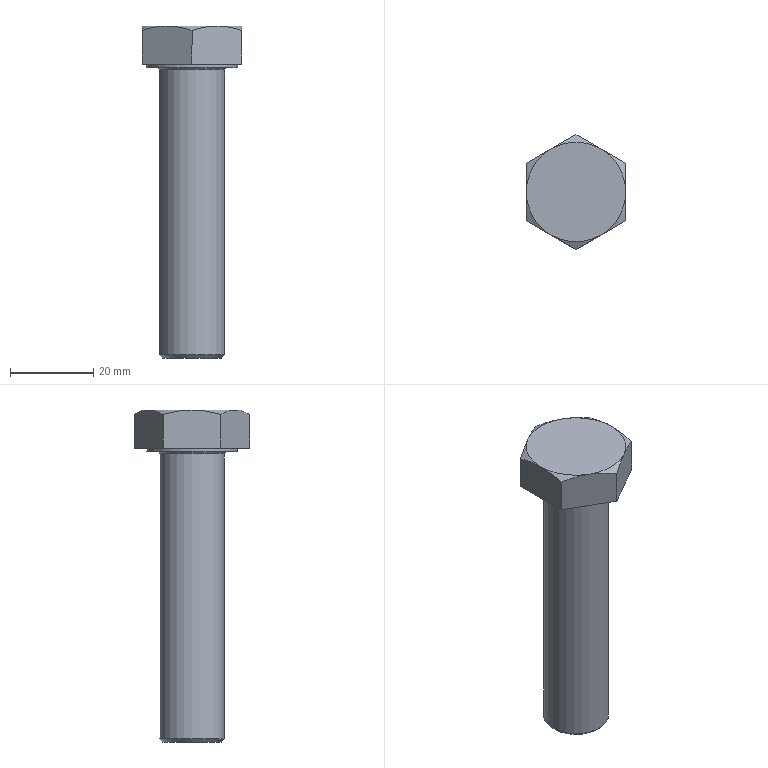Part | NX | features SKETCH 4, EXTRUDE 3, META 3, DATUM_CSYS 2, BLEND 1, CHAMFER 1, LINE 1, SWP104 1, SYMBOLIC_THREAD 1, THREADS 1 | 1 solid | 20 faces | box 24 x 27.713 x 80 mm | volume 18388 mm3 | plane 10 | cone 7 | cylinder 2 | torus 1 | commonest cylinder face diameters 15.682 x1 22 x1
STEP:
#1=CARTESIAN_POINT('',(8.441,0.,0.));
#2=VERTEX_POINT('',#1);
#3=CARTESIAN_POINT('',(0.,0.,0.));
#4=DIRECTION('',(0.,0.,1.));
#5=DIRECTION('',(1.,0.,0.));
#6=AXIS2_PLACEMENT_3D('',#3,#4,#5);
#7=CIRCLE('',#6,8.441);
#8=EDGE_CURVE('',#2,#2,#7,.T.);
#9=ORIENTED_EDGE('',*,*,#8,.T.);
#10=EDGE_LOOP('',(#9));
#11=FACE_BOUND('',#10,.T.);
#12=CARTESIAN_POINT('',(11.,0.,0.));
#13=VERTEX_POINT('',#12);
#14=CARTESIAN_POINT('',(0.,0.,0.));
#15=DIRECTION('',(0.,0.,1.));
#16=DIRECTION('',(1.,0.,0.));
#17=AXIS2_PLACEMENT_3D('',#14,#15,#16);
#18=CIRCLE('',#17,11.);
#19=EDGE_CURVE('',#13,#13,#18,.T.);
#20=ORIENTED_EDGE('',*,*,#19,.F.);
#21=EDGE_LOOP('',(#20));
#22=FACE_BOUND('',#21,.T.);
#23=CARTESIAN_POINT('',(0.,0.,0.));
#24=DIRECTION('',(0.,0.,1.));
#25=DIRECTION('',(1.,0.,0.));
#26=AXIS2_PLACEMENT_3D('',#23,#24,#25);
#27=PLANE('',#26);
#28=ADVANCED_FACE('',(#11,#22),#27,.F.);
#29=CARTESIAN_POINT('',(12.,6.928,8.928));
#30=VERTEX_POINT('',#29);
#31=CARTESIAN_POINT('',(6.,10.392,10.));
#32=VERTEX_POINT('',#31);
#33=CARTESIAN_POINT('',(12.,6.928,8.928));
#34=CARTESIAN_POINT('',(10.037,8.062,9.583));
#35=CARTESIAN_POINT('',(8.044,9.212,10.));
#36=CARTESIAN_POINT('',(6.,10.392,10.));
#37=B_SPLINE_CURVE_WITH_KNOTS('',3,(#33,#34,#35,#36),.UNSPECIFIED.,.F.,.F.,(4,4),(0.000000238,0.00701),.UNSPECIFIED.);
#38=EDGE_CURVE('',#30,#32,#37,.T.);
#39=ORIENTED_EDGE('',*,*,#38,.F.);
#40=CARTESIAN_POINT('',(12.,6.928,0.8));
#41=VERTEX_POINT('',#40);
#42=CARTESIAN_POINT('',(12.,6.928,10.));
#43=DIRECTION('',(0.,0.,-1.));
#44=VECTOR('',#43,1000.);
#45=LINE('',#42,#44);
#46=EDGE_CURVE('',#30,#41,#45,.T.);
#47=ORIENTED_EDGE('',*,*,#46,.T.);
#48=CARTESIAN_POINT('',(0.,13.856,0.8));
#49=VERTEX_POINT('',#48);
#50=CARTESIAN_POINT('',(0.,13.856,0.8));
#51=DIRECTION('',(0.866,-0.5,0.));
#52=VECTOR('',#51,1000.);
#53=LINE('',#50,#52);
#54=EDGE_CURVE('',#49,#41,#53,.T.);
#55=ORIENTED_EDGE('',*,*,#54,.F.);
#56=CARTESIAN_POINT('',(0.,13.856,8.928));
#57=VERTEX_POINT('',#56);
#58=CARTESIAN_POINT('',(0.,13.856,10.));
#59=DIRECTION('',(0.,0.,-1.));
#60=VECTOR('',#59,1000.);
#61=LINE('',#58,#60);
#62=EDGE_CURVE('',#57,#49,#61,.T.);
#63=ORIENTED_EDGE('',*,*,#62,.F.);
#64=CARTESIAN_POINT('',(6.,10.392,10.));
#65=CARTESIAN_POINT('',(3.963,11.568,10.));
#66=CARTESIAN_POINT('',(1.958,12.726,9.581));
#67=CARTESIAN_POINT('',(0.,13.856,8.928));
#68=B_SPLINE_CURVE_WITH_KNOTS('',3,(#64,#65,#66,#67),.UNSPECIFIED.,.F.,.F.,(4,4),(0.00701,0.01399),.UNSPECIFIED.);
#69=EDGE_CURVE('',#32,#57,#68,.T.);
#70=ORIENTED_EDGE('',*,*,#69,.F.);
#71=EDGE_LOOP('',(#39,#47,#55,#63,#70));
#72=FACE_BOUND('',#71,.T.);
#73=CARTESIAN_POINT('',(0.,13.856,10.));
#74=DIRECTION('',(0.5,0.866,0.));
#75=DIRECTION('',(-0.866,0.5,0.));
#76=AXIS2_PLACEMENT_3D('',#73,#74,#75);
#77=PLANE('',#76);
#78=ADVANCED_FACE('',(#72),#77,.T.);
#79=CARTESIAN_POINT('',(12.,-6.928,8.928));
#80=VERTEX_POINT('',#79);
#81=CARTESIAN_POINT('',(12.,0.,10.));
#82=VERTEX_POINT('',#81);
#83=CARTESIAN_POINT('',(12.,-6.928,8.928));
#84=CARTESIAN_POINT('',(12.,-4.675,9.579));
#85=CARTESIAN_POINT('',(12.,-2.342,10.));
#86=CARTESIAN_POINT('',(12.,0.,10.));
#87=B_SPLINE_CURVE_WITH_KNOTS('',3,(#83,#84,#85,#86),.UNSPECIFIED.,.F.,.F.,(4,4),(0.01236,0.01937),.UNSPECIFIED.);
#88=EDGE_CURVE('',#80,#82,#87,.T.);
#89=ORIENTED_EDGE('',*,*,#88,.F.);
#90=CARTESIAN_POINT('',(12.,-6.928,0.8));
#91=VERTEX_POINT('',#90);
#92=CARTESIAN_POINT('',(12.,-6.928,10.));
#93=DIRECTION('',(0.,0.,-1.));
#94=VECTOR('',#93,1000.);
#95=LINE('',#92,#94);
#96=EDGE_CURVE('',#80,#91,#95,.T.);
#97=ORIENTED_EDGE('',*,*,#96,.T.);
#98=CARTESIAN_POINT('',(12.,6.928,0.8));
#99=DIRECTION('',(0.,-1.,0.));
#100=VECTOR('',#99,1000.);
#101=LINE('',#98,#100);
#102=EDGE_CURVE('',#41,#91,#101,.T.);
#103=ORIENTED_EDGE('',*,*,#102,.F.);
#104=ORIENTED_EDGE('',*,*,#46,.F.);
#105=CARTESIAN_POINT('',(12.,0.,10.));
#106=CARTESIAN_POINT('',(12.,2.343,10.));
#107=CARTESIAN_POINT('',(12.,4.688,9.575));
#108=CARTESIAN_POINT('',(12.,6.928,8.928));
#109=B_SPLINE_CURVE_WITH_KNOTS('',3,(#105,#106,#107,#108),.UNSPECIFIED.,.F.,.F.,(4,4),(0.01937,0.02638),.UNSPECIFIED.);
#110=EDGE_CURVE('',#82,#30,#109,.T.);
#111=ORIENTED_EDGE('',*,*,#110,.F.);
#112=EDGE_LOOP('',(#89,#97,#103,#104,#111));
#113=FACE_BOUND('',#112,.T.);
#114=CARTESIAN_POINT('',(12.,6.928,10.));
#115=DIRECTION('',(1.,0.,0.));
#116=DIRECTION('',(0.,0.,-1.));
#117=AXIS2_PLACEMENT_3D('',#114,#115,#116);
#118=PLANE('',#117);
#119=ADVANCED_FACE('',(#113),#118,.T.);
#120=CARTESIAN_POINT('',(0.,-13.856,8.928));
#121=VERTEX_POINT('',#120);
#122=CARTESIAN_POINT('',(6.,-10.392,10.));
#123=VERTEX_POINT('',#122);
#124=CARTESIAN_POINT('',(0.,-13.856,8.928));
#125=CARTESIAN_POINT('',(1.963,-12.723,9.583));
#126=CARTESIAN_POINT('',(3.956,-11.573,10.));
#127=CARTESIAN_POINT('',(6.,-10.392,10.));
#128=B_SPLINE_CURVE_WITH_KNOTS('',3,(#124,#125,#126,#127),.UNSPECIFIED.,.F.,.F.,(4,4),(0.000000238,0.00701),.UNSPECIFIED.);
#129=EDGE_CURVE('',#121,#123,#128,.T.);
#130=ORIENTED_EDGE('',*,*,#129,.F.);
#131=CARTESIAN_POINT('',(0.,-13.856,0.8));
#132=VERTEX_POINT('',#131);
#133=CARTESIAN_POINT('',(0.,-13.856,10.));
#134=DIRECTION('',(0.,0.,-1.));
#135=VECTOR('',#134,1000.);
#136=LINE('',#133,#135);
#137=EDGE_CURVE('',#121,#132,#136,.T.);
#138=ORIENTED_EDGE('',*,*,#137,.T.);
#139=CARTESIAN_POINT('',(12.,-6.928,0.8));
#140=DIRECTION('',(-0.866,-0.5,0.));
#141=VECTOR('',#140,1000.);
#142=LINE('',#139,#141);
#143=EDGE_CURVE('',#91,#132,#142,.T.);
#144=ORIENTED_EDGE('',*,*,#143,.F.);
#145=ORIENTED_EDGE('',*,*,#96,.F.);
#146=CARTESIAN_POINT('',(6.,-10.392,10.));
#147=CARTESIAN_POINT('',(8.037,-9.216,10.));
#148=CARTESIAN_POINT('',(10.042,-8.059,9.581));
#149=CARTESIAN_POINT('',(12.,-6.928,8.928));
#150=B_SPLINE_CURVE_WITH_KNOTS('',3,(#146,#147,#148,#149),.UNSPECIFIED.,.F.,.F.,(4,4),(0.00701,0.01399),.UNSPECIFIED.);
#151=EDGE_CURVE('',#123,#80,#150,.T.);
#152=ORIENTED_EDGE('',*,*,#151,.F.);
#153=EDGE_LOOP('',(#130,#138,#144,#145,#152));
#154=FACE_BOUND('',#153,.T.);
#155=CARTESIAN_POINT('',(12.,-6.928,10.));
#156=DIRECTION('',(0.5,-0.866,0.));
#157=DIRECTION('',(0.866,0.5,0.));
#158=AXIS2_PLACEMENT_3D('',#155,#156,#157);
#159=PLANE('',#158);
#160=ADVANCED_FACE('',(#154),#159,.T.);
#161=CARTESIAN_POINT('',(-12.,-6.928,8.928));
#162=VERTEX_POINT('',#161);
#163=CARTESIAN_POINT('',(-6.,-10.392,10.));
#164=VERTEX_POINT('',#163);
#165=CARTESIAN_POINT('',(-12.,-6.928,8.928));
#166=CARTESIAN_POINT('',(-10.037,-8.062,9.583));
#167=CARTESIAN_POINT('',(-8.044,-9.212,10.));
#168=CARTESIAN_POINT('',(-6.,-10.392,10.));
#169=B_SPLINE_CURVE_WITH_KNOTS('',3,(#165,#166,#167,#168),.UNSPECIFIED.,.F.,.F.,(4,4),(0.000000238,0.00701),.UNSPECIFIED.);
#170=EDGE_CURVE('',#162,#164,#169,.T.);
#171=ORIENTED_EDGE('',*,*,#170,.F.);
#172=CARTESIAN_POINT('',(-12.,-6.928,0.8));
#173=VERTEX_POINT('',#172);
#174=CARTESIAN_POINT('',(-12.,-6.928,10.));
#175=DIRECTION('',(0.,0.,-1.));
#176=VECTOR('',#175,1000.);
#177=LINE('',#174,#176);
#178=EDGE_CURVE('',#162,#173,#177,.T.);
#179=ORIENTED_EDGE('',*,*,#178,.T.);
#180=CARTESIAN_POINT('',(0.,-13.856,0.8));
#181=DIRECTION('',(-0.866,0.5,0.));
#182=VECTOR('',#181,1000.);
#183=LINE('',#180,#182);
#184=EDGE_CURVE('',#132,#173,#183,.T.);
#185=ORIENTED_EDGE('',*,*,#184,.F.);
#186=ORIENTED_EDGE('',*,*,#137,.F.);
#187=CARTESIAN_POINT('',(-6.,-10.392,10.));
#188=CARTESIAN_POINT('',(-3.963,-11.568,10.));
#189=CARTESIAN_POINT('',(-1.958,-12.726,9.581));
#190=CARTESIAN_POINT('',(0.,-13.856,8.928));
#191=B_SPLINE_CURVE_WITH_KNOTS('',3,(#187,#188,#189,#190),.UNSPECIFIED.,.F.,.F.,(4,4),(0.00701,0.01399),.UNSPECIFIED.);
#192=EDGE_CURVE('',#164,#121,#191,.T.);
#193=ORIENTED_EDGE('',*,*,#192,.F.);
#194=EDGE_LOOP('',(#171,#179,#185,#186,#193));
#195=FACE_BOUND('',#194,.T.);
#196=CARTESIAN_POINT('',(0.,-13.856,10.));
#197=DIRECTION('',(-0.5,-0.866,0.));
#198=DIRECTION('',(0.866,-0.5,0.));
#199=AXIS2_PLACEMENT_3D('',#196,#197,#198);
#200=PLANE('',#199);
#201=ADVANCED_FACE('',(#195),#200,.T.);
#202=CARTESIAN_POINT('',(-12.,6.928,8.928));
#203=VERTEX_POINT('',#202);
#204=CARTESIAN_POINT('',(-12.,0.,10.));
#205=VERTEX_POINT('',#204);
#206=CARTESIAN_POINT('',(-12.,0.,10.));
#207=CARTESIAN_POINT('',(-12.,2.343,10.));
#208=CARTESIAN_POINT('',(-12.,4.688,9.575));
#209=CARTESIAN_POINT('',(-12.,6.928,8.928));
#210=B_SPLINE_CURVE_WITH_KNOTS('',3,(#206,#207,#208,#209),.UNSPECIFIED.,.F.,.F.,(4,4),(0.01937,0.02638),.UNSPECIFIED.);
#211=EDGE_CURVE('',#203,#205,#210,.F.);
#212=ORIENTED_EDGE('',*,*,#211,.F.);
#213=CARTESIAN_POINT('',(-12.,6.928,0.8));
#214=VERTEX_POINT('',#213);
#215=CARTESIAN_POINT('',(-12.,6.928,10.));
#216=DIRECTION('',(0.,0.,-1.));
#217=VECTOR('',#216,1000.);
#218=LINE('',#215,#217);
#219=EDGE_CURVE('',#203,#214,#218,.T.);
#220=ORIENTED_EDGE('',*,*,#219,.T.);
#221=CARTESIAN_POINT('',(-12.,-6.928,0.8));
#222=DIRECTION('',(0.,1.,0.));
#223=VECTOR('',#222,1000.);
#224=LINE('',#221,#223);
#225=EDGE_CURVE('',#173,#214,#224,.T.);
#226=ORIENTED_EDGE('',*,*,#225,.F.);
#227=ORIENTED_EDGE('',*,*,#178,.F.);
#228=CARTESIAN_POINT('',(-12.,-6.928,8.928));
#229=CARTESIAN_POINT('',(-12.,-4.675,9.579));
#230=CARTESIAN_POINT('',(-12.,-2.342,10.));
#231=CARTESIAN_POINT('',(-12.,0.,10.));
#232=B_SPLINE_CURVE_WITH_KNOTS('',3,(#228,#229,#230,#231),.UNSPECIFIED.,.F.,.F.,(4,4),(0.01236,0.01937),.UNSPECIFIED.);
#233=EDGE_CURVE('',#205,#162,#232,.F.);
#234=ORIENTED_EDGE('',*,*,#233,.F.);
#235=EDGE_LOOP('',(#212,#220,#226,#227,#234));
#236=FACE_BOUND('',#235,.T.);
#237=CARTESIAN_POINT('',(-12.,-6.928,10.));
#238=DIRECTION('',(-1.,0.,0.));
#239=DIRECTION('',(0.,0.,1.));
#240=AXIS2_PLACEMENT_3D('',#237,#238,#239);
#241=PLANE('',#240);
#242=ADVANCED_FACE('',(#236),#241,.T.);
#243=CARTESIAN_POINT('',(-6.,10.392,10.));
#244=VERTEX_POINT('',#243);
#245=CARTESIAN_POINT('',(0.,13.856,8.928));
#246=CARTESIAN_POINT('',(-1.963,12.723,9.583));
#247=CARTESIAN_POINT('',(-3.956,11.573,10.));
#248=CARTESIAN_POINT('',(-6.,10.392,10.));
#249=B_SPLINE_CURVE_WITH_KNOTS('',3,(#245,#246,#247,#248),.UNSPECIFIED.,.F.,.F.,(4,4),(0.000000238,0.00701),.UNSPECIFIED.);
#250=EDGE_CURVE('',#57,#244,#249,.T.);
#251=ORIENTED_EDGE('',*,*,#250,.F.);
#252=ORIENTED_EDGE('',*,*,#62,.T.);
#253=CARTESIAN_POINT('',(-12.,6.928,0.8));
#254=DIRECTION('',(0.866,0.5,0.));
#255=VECTOR('',#254,1000.);
#256=LINE('',#253,#255);
#257=EDGE_CURVE('',#214,#49,#256,.T.);
#258=ORIENTED_EDGE('',*,*,#257,.F.);
#259=ORIENTED_EDGE('',*,*,#219,.F.);
#260=CARTESIAN_POINT('',(-6.,10.392,10.));
#261=CARTESIAN_POINT('',(-8.037,9.216,10.));
#262=CARTESIAN_POINT('',(-10.042,8.059,9.581));
#263=CARTESIAN_POINT('',(-12.,6.928,8.928));
#264=B_SPLINE_CURVE_WITH_KNOTS('',3,(#260,#261,#262,#263),.UNSPECIFIED.,.F.,.F.,(4,4),(0.00701,0.01399),.UNSPECIFIED.);
#265=EDGE_CURVE('',#244,#203,#264,.T.);
#266=ORIENTED_EDGE('',*,*,#265,.F.);
#267=EDGE_LOOP('',(#251,#252,#258,#259,#266));
#268=FACE_BOUND('',#267,.T.);
#269=CARTESIAN_POINT('',(-12.,6.928,10.));
#270=DIRECTION('',(-0.5,0.866,0.));
#271=DIRECTION('',(-0.866,-0.5,0.));
#272=AXIS2_PLACEMENT_3D('',#269,#270,#271);
#273=PLANE('',#272);
#274=ADVANCED_FACE('',(#268),#273,.T.);
#275=CARTESIAN_POINT('',(11.,0.,0.8));
#276=VERTEX_POINT('',#275);
#277=CARTESIAN_POINT('',(0.,0.,0.8));
#278=DIRECTION('',(0.,0.,1.));
#279=DIRECTION('',(1.,0.,0.));
#280=AXIS2_PLACEMENT_3D('',#277,#278,#279);
#281=CIRCLE('',#280,11.);
#282=EDGE_CURVE('',#276,#276,#281,.T.);
#283=ORIENTED_EDGE('',*,*,#282,.T.);
#284=EDGE_LOOP('',(#283));
#285=FACE_BOUND('',#284,.T.);
#286=ORIENTED_EDGE('',*,*,#54,.T.);
#287=ORIENTED_EDGE('',*,*,#102,.T.);
#288=ORIENTED_EDGE('',*,*,#143,.T.);
#289=ORIENTED_EDGE('',*,*,#184,.T.);
#290=ORIENTED_EDGE('',*,*,#225,.T.);
#291=ORIENTED_EDGE('',*,*,#257,.T.);
#292=EDGE_LOOP('',(#286,#287,#288,#289,#290,#291));
#293=FACE_BOUND('',#292,.T.);
#294=CARTESIAN_POINT('',(0.,13.856,0.8));
#295=DIRECTION('',(0.,0.,1.));
#296=DIRECTION('',(1.,0.,0.));
#297=AXIS2_PLACEMENT_3D('',#294,#295,#296);
#298=PLANE('',#297);
#299=ADVANCED_FACE('',(#285,#293),#298,.F.);
#300=ORIENTED_EDGE('',*,*,#282,.F.);
#301=EDGE_LOOP('',(#300));
#302=FACE_BOUND('',#301,.T.);
#303=ORIENTED_EDGE('',*,*,#19,.T.);
#304=EDGE_LOOP('',(#303));
#305=FACE_BOUND('',#304,.T.);
#306=CARTESIAN_POINT('',(0.,0.,0.8));
#307=DIRECTION('',(0.,0.,-1.));
#308=DIRECTION('',(-1.,0.,0.));
#309=AXIS2_PLACEMENT_3D('',#306,#307,#308);
#310=CYLINDRICAL_SURFACE('',#309,11.);
#311=ADVANCED_FACE('',(#302,#305),#310,.T.);
#312=CARTESIAN_POINT('',(-7.841,0.,-69.216));
#313=VERTEX_POINT('',#312);
#314=CARTESIAN_POINT('',(0.,0.,-69.216));
#315=DIRECTION('',(0.,0.,-1.));
#316=DIRECTION('',(-1.,0.,0.));
#317=AXIS2_PLACEMENT_3D('',#314,#315,#316);
#318=CIRCLE('',#317,7.841);
#319=EDGE_CURVE('',#313,#313,#318,.F.);
#320=ORIENTED_EDGE('',*,*,#319,.T.);
#321=EDGE_LOOP('',(#320));
#322=FACE_BOUND('',#321,.T.);
#323=CARTESIAN_POINT('',(7.841,0.,-0.6));
#324=VERTEX_POINT('',#323);
#325=CARTESIAN_POINT('',(0.,0.,-0.6));
#326=DIRECTION('',(0.,0.,1.));
#327=DIRECTION('',(1.,0.,0.));
#328=AXIS2_PLACEMENT_3D('',#325,#326,#327);
#329=CIRCLE('',#328,7.841);
#330=EDGE_CURVE('',#324,#324,#329,.F.);
#331=ORIENTED_EDGE('',*,*,#330,.T.);
#332=EDGE_LOOP('',(#331));
#333=FACE_BOUND('',#332,.T.);
#334=CARTESIAN_POINT('',(0.,0.,-70.));
#335=DIRECTION('',(0.,0.,1.));
#336=DIRECTION('',(1.,0.,0.));
#337=AXIS2_PLACEMENT_3D('',#334,#335,#336);
#338=CYLINDRICAL_SURFACE('',#337,7.841);
#339=ADVANCED_FACE('',(#322,#333),#338,.T.);
#340=CARTESIAN_POINT('',(-7.057,0.,-70.));
#341=VERTEX_POINT('',#340);
#342=CARTESIAN_POINT('',(0.,0.,-70.));
#343=DIRECTION('',(0.,0.,-1.));
#344=DIRECTION('',(-1.,0.,0.));
#345=AXIS2_PLACEMENT_3D('',#342,#343,#344);
#346=CIRCLE('',#345,7.057);
#347=EDGE_CURVE('',#341,#341,#346,.T.);
#348=ORIENTED_EDGE('',*,*,#347,.T.);
#349=EDGE_LOOP('',(#348));
#350=FACE_BOUND('',#349,.T.);
#351=CARTESIAN_POINT('',(0.,0.,-70.));
#352=DIRECTION('',(0.,0.,-1.));
#353=DIRECTION('',(-1.,0.,0.));
#354=AXIS2_PLACEMENT_3D('',#351,#352,#353);
#355=PLANE('',#354);
#356=ADVANCED_FACE('',(#350),#355,.T.);
#357=ORIENTED_EDGE('',*,*,#211,.T.);
#358=CARTESIAN_POINT('',(0.,0.,10.));
#359=DIRECTION('',(0.,0.,-1.));
#360=DIRECTION('',(-1.,0.,0.));
#361=AXIS2_PLACEMENT_3D('',#358,#359,#360);
#362=CIRCLE('',#361,12.);
#363=EDGE_CURVE('',#205,#244,#362,.T.);
#364=ORIENTED_EDGE('',*,*,#363,.T.);
#365=ORIENTED_EDGE('',*,*,#265,.T.);
#366=EDGE_LOOP('',(#357,#364,#365));
#367=FACE_BOUND('',#366,.T.);
#368=CARTESIAN_POINT('',(0.,0.,10.));
#369=DIRECTION('',(0.,0.,-1.));
#370=DIRECTION('',(-1.,0.,0.));
#371=AXIS2_PLACEMENT_3D('',#368,#369,#370);
#372=CONICAL_SURFACE('',#371,12.,1.047);
#373=ADVANCED_FACE('',(#367),#372,.T.);
#374=ORIENTED_EDGE('',*,*,#69,.T.);
#375=ORIENTED_EDGE('',*,*,#250,.T.);
#376=CARTESIAN_POINT('',(0.,0.,10.));
#377=DIRECTION('',(0.,0.,-1.));
#378=DIRECTION('',(-1.,0.,0.));
#379=AXIS2_PLACEMENT_3D('',#376,#377,#378);
#380=CIRCLE('',#379,12.);
#381=EDGE_CURVE('',#244,#32,#380,.T.);
#382=ORIENTED_EDGE('',*,*,#381,.T.);
#383=EDGE_LOOP('',(#374,#375,#382));
#384=FACE_BOUND('',#383,.T.);
#385=CARTESIAN_POINT('',(0.,0.,10.));
#386=DIRECTION('',(0.,0.,-1.));
#387=DIRECTION('',(-1.,0.,0.));
#388=AXIS2_PLACEMENT_3D('',#385,#386,#387);
#389=CONICAL_SURFACE('',#388,12.,1.047);
#390=ADVANCED_FACE('',(#384),#389,.T.);
#391=ORIENTED_EDGE('',*,*,#170,.T.);
#392=CARTESIAN_POINT('',(0.,0.,10.));
#393=DIRECTION('',(0.,0.,-1.));
#394=DIRECTION('',(-1.,0.,0.));
#395=AXIS2_PLACEMENT_3D('',#392,#393,#394);
#396=CIRCLE('',#395,12.);
#397=EDGE_CURVE('',#164,#205,#396,.T.);
#398=ORIENTED_EDGE('',*,*,#397,.T.);
#399=ORIENTED_EDGE('',*,*,#233,.T.);
#400=EDGE_LOOP('',(#391,#398,#399));
#401=FACE_BOUND('',#400,.T.);
#402=CARTESIAN_POINT('',(0.,0.,10.));
#403=DIRECTION('',(0.,0.,-1.));
#404=DIRECTION('',(-1.,0.,0.));
#405=AXIS2_PLACEMENT_3D('',#402,#403,#404);
#406=CONICAL_SURFACE('',#405,12.,1.047);
#407=ADVANCED_FACE('',(#401),#406,.T.);
#408=ORIENTED_EDGE('',*,*,#129,.T.);
#409=CARTESIAN_POINT('',(0.,0.,10.));
#410=DIRECTION('',(0.,0.,-1.));
#411=DIRECTION('',(-1.,0.,0.));
#412=AXIS2_PLACEMENT_3D('',#409,#410,#411);
#413=CIRCLE('',#412,12.);
#414=EDGE_CURVE('',#123,#164,#413,.T.);
#415=ORIENTED_EDGE('',*,*,#414,.T.);
#416=ORIENTED_EDGE('',*,*,#192,.T.);
#417=EDGE_LOOP('',(#408,#415,#416));
#418=FACE_BOUND('',#417,.T.);
#419=CARTESIAN_POINT('',(0.,0.,10.));
#420=DIRECTION('',(0.,0.,-1.));
#421=DIRECTION('',(-1.,0.,0.));
#422=AXIS2_PLACEMENT_3D('',#419,#420,#421);
#423=CONICAL_SURFACE('',#422,12.,1.047);
#424=ADVANCED_FACE('',(#418),#423,.T.);
#425=ORIENTED_EDGE('',*,*,#151,.T.);
#426=ORIENTED_EDGE('',*,*,#88,.T.);
#427=CARTESIAN_POINT('',(0.,0.,10.));
#428=DIRECTION('',(0.,0.,-1.));
#429=DIRECTION('',(-1.,0.,0.));
#430=AXIS2_PLACEMENT_3D('',#427,#428,#429);
#431=CIRCLE('',#430,12.);
#432=EDGE_CURVE('',#82,#123,#431,.T.);
#433=ORIENTED_EDGE('',*,*,#432,.T.);
#434=EDGE_LOOP('',(#425,#426,#433));
#435=FACE_BOUND('',#434,.T.);
#436=CARTESIAN_POINT('',(0.,0.,10.));
#437=DIRECTION('',(0.,0.,-1.));
#438=DIRECTION('',(-1.,0.,0.));
#439=AXIS2_PLACEMENT_3D('',#436,#437,#438);
#440=CONICAL_SURFACE('',#439,12.,1.047);
#441=ADVANCED_FACE('',(#435),#440,.T.);
#442=ORIENTED_EDGE('',*,*,#110,.T.);
#443=ORIENTED_EDGE('',*,*,#38,.T.);
#444=CARTESIAN_POINT('',(0.,0.,10.));
#445=DIRECTION('',(0.,0.,-1.));
#446=DIRECTION('',(-1.,0.,0.));
#447=AXIS2_PLACEMENT_3D('',#444,#445,#446);
#448=CIRCLE('',#447,12.);
#449=EDGE_CURVE('',#32,#82,#448,.T.);
#450=ORIENTED_EDGE('',*,*,#449,.T.);
#451=EDGE_LOOP('',(#442,#443,#450));
#452=FACE_BOUND('',#451,.T.);
#453=CARTESIAN_POINT('',(0.,0.,10.));
#454=DIRECTION('',(0.,0.,-1.));
#455=DIRECTION('',(-1.,0.,0.));
#456=AXIS2_PLACEMENT_3D('',#453,#454,#455);
#457=CONICAL_SURFACE('',#456,12.,1.047);
#458=ADVANCED_FACE('',(#452),#457,.T.);
#459=ORIENTED_EDGE('',*,*,#363,.F.);
#460=ORIENTED_EDGE('',*,*,#397,.F.);
#461=ORIENTED_EDGE('',*,*,#414,.F.);
#462=ORIENTED_EDGE('',*,*,#432,.F.);
#463=ORIENTED_EDGE('',*,*,#449,.F.);
#464=ORIENTED_EDGE('',*,*,#381,.F.);
#465=EDGE_LOOP('',(#459,#460,#461,#462,#463,#464));
#466=FACE_BOUND('',#465,.T.);
#467=CARTESIAN_POINT('',(0.,13.856,10.));
#468=DIRECTION('',(0.,0.,1.));
#469=DIRECTION('',(1.,0.,0.));
#470=AXIS2_PLACEMENT_3D('',#467,#468,#469);
#471=PLANE('',#470);
#472=ADVANCED_FACE('',(#466),#471,.T.);
#473=ORIENTED_EDGE('',*,*,#8,.F.);
#474=EDGE_LOOP('',(#473));
#475=FACE_BOUND('',#474,.T.);
#476=ORIENTED_EDGE('',*,*,#330,.F.);
#477=EDGE_LOOP('',(#476));
#478=FACE_BOUND('',#477,.T.);
#479=CARTESIAN_POINT('',(0.,0.,-0.6));
#480=DIRECTION('',(0.,0.,1.));
#481=DIRECTION('',(1.,0.,0.));
#482=AXIS2_PLACEMENT_3D('',#479,#480,#481);
#483=TOROIDAL_SURFACE('',#482,8.441,0.6);
#484=ADVANCED_FACE('',(#475,#478),#483,.F.);
#485=ORIENTED_EDGE('',*,*,#319,.F.);
#486=EDGE_LOOP('',(#485));
#487=FACE_BOUND('',#486,.T.);
#488=ORIENTED_EDGE('',*,*,#347,.F.);
#489=EDGE_LOOP('',(#488));
#490=FACE_BOUND('',#489,.T.);
#491=CARTESIAN_POINT('',(0.,0.,-70.));
#492=DIRECTION('',(0.,0.,1.));
#493=DIRECTION('',(1.,0.,0.));
#494=AXIS2_PLACEMENT_3D('',#491,#492,#493);
#495=CONICAL_SURFACE('',#494,7.057,0.7854);
#496=ADVANCED_FACE('',(#487,#490),#495,.T.);
#497=CLOSED_SHELL('',(#28,#78,#119,#160,#201,#242,#274,#299,#311,#339,#356,#373,#390,#407,#424,#441,#458,#472,#484,#496));
#498=MANIFOLD_SOLID_BREP('',#497);
#499=(LENGTH_UNIT()NAMED_UNIT(*)SI_UNIT(.MILLI.,.METRE.));
#500=UNCERTAINTY_MEASURE_WITH_UNIT(LENGTH_MEASURE(0.0508),#499,'','');
#501=(NAMED_UNIT(*)PLANE_ANGLE_UNIT()SI_UNIT($,.RADIAN.));
#502=(NAMED_UNIT(*)SI_UNIT($,.STERADIAN.)SOLID_ANGLE_UNIT());
#503=(GEOMETRIC_REPRESENTATION_CONTEXT(3)GLOBAL_UNCERTAINTY_ASSIGNED_CONTEXT((#500))GLOBAL_UNIT_ASSIGNED_CONTEXT((#499,#501,#502))REPRESENTATION_CONTEXT('',''));
#504=ADVANCED_BREP_SHAPE_REPRESENTATION('',(#498),#503);